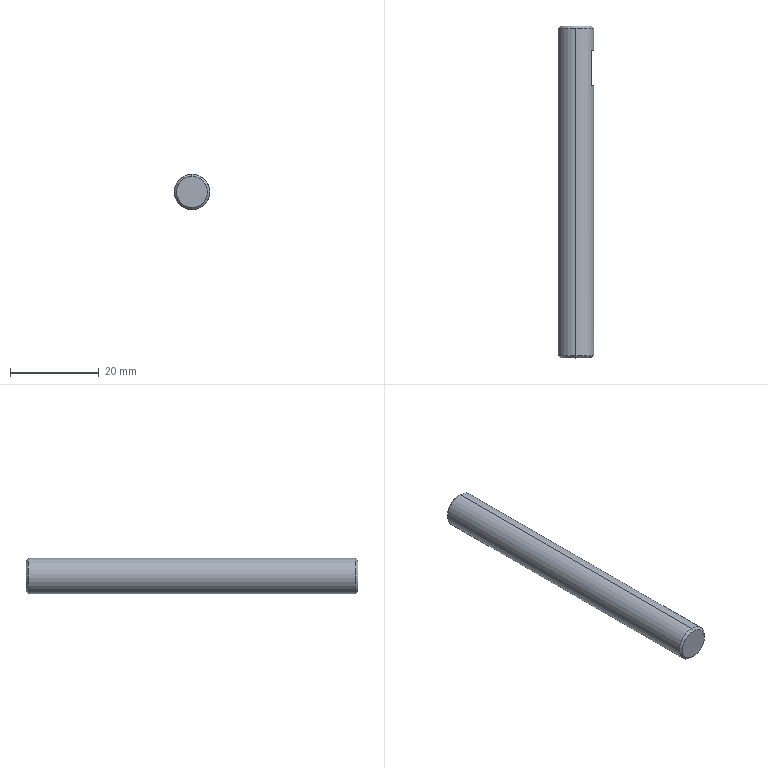Part | SolidWorks | features Chamfer 1, Extrusion 1, ICE 1 | 1 solid | 11 faces | box 8 x 75 x 8 mm | volume 3753 mm3 | plane 5 | cone 4 | cylinder 2 | commonest cylinder face diameters 8 x2
STEP:
#1=CARTESIAN_POINT('',(0.,75.,3.5));
#2=VERTEX_POINT('',#1);
#3=CARTESIAN_POINT('',(0.,75.,-3.5));
#4=VERTEX_POINT('',#3);
#5=CARTESIAN_POINT('',(0.,75.,0.));
#6=DIRECTION('',(0.,1.,0.));
#7=DIRECTION('',(0.,0.,1.));
#8=AXIS2_PLACEMENT_3D('',#5,#6,#7);
#9=CIRCLE('',#8,3.5);
#10=EDGE_CURVE('',#2,#4,#9,.T.);
#11=ORIENTED_EDGE('',*,*,#10,.F.);
#12=CARTESIAN_POINT('',(0.,74.5,4.));
#13=VERTEX_POINT('',#12);
#14=CARTESIAN_POINT('',(0.,75.,3.5));
#15=DIRECTION('',(0.,-0.7071,0.7071));
#16=VECTOR('',#15,1000.);
#17=LINE('',#14,#16);
#18=EDGE_CURVE('',#2,#13,#17,.T.);
#19=ORIENTED_EDGE('',*,*,#18,.T.);
#20=CARTESIAN_POINT('',(0.,74.5,-4.));
#21=VERTEX_POINT('',#20);
#22=CARTESIAN_POINT('',(0.,74.5,0.));
#23=DIRECTION('',(0.,-1.,0.));
#24=DIRECTION('',(0.,0.,1.));
#25=AXIS2_PLACEMENT_3D('',#22,#23,#24);
#26=CIRCLE('',#25,4.);
#27=EDGE_CURVE('',#21,#13,#26,.T.);
#28=ORIENTED_EDGE('',*,*,#27,.F.);
#29=CARTESIAN_POINT('',(0.,75.,-3.5));
#30=DIRECTION('',(0.,-0.7071,-0.7071));
#31=VECTOR('',#30,1000.);
#32=LINE('',#29,#31);
#33=EDGE_CURVE('',#4,#21,#32,.T.);
#34=ORIENTED_EDGE('',*,*,#33,.F.);
#35=EDGE_LOOP('',(#11,#19,#28,#34));
#36=FACE_OUTER_BOUND('',#35,.T.);
#37=CARTESIAN_POINT('',(0.,75.,0.));
#38=DIRECTION('',(0.,-1.,0.));
#39=DIRECTION('',(0.,0.,-1.));
#40=AXIS2_PLACEMENT_3D('',#37,#38,#39);
#41=CONICAL_SURFACE('',#40,3.5,0.7854);
#42=ADVANCED_FACE('',(#36),#41,.T.);
#43=CARTESIAN_POINT('',(0.,0.,-3.5));
#44=VERTEX_POINT('',#43);
#45=CARTESIAN_POINT('',(0.,0.,3.5));
#46=VERTEX_POINT('',#45);
#47=CARTESIAN_POINT('',(0.,0.,0.));
#48=DIRECTION('',(0.,-1.,0.));
#49=DIRECTION('',(0.,0.,1.));
#50=AXIS2_PLACEMENT_3D('',#47,#48,#49);
#51=CIRCLE('',#50,3.5);
#52=EDGE_CURVE('',#44,#46,#51,.T.);
#53=ORIENTED_EDGE('',*,*,#52,.F.);
#54=CARTESIAN_POINT('',(0.,0.5,-4.));
#55=VERTEX_POINT('',#54);
#56=CARTESIAN_POINT('',(0.,0.5,-4.));
#57=DIRECTION('',(0.,0.7071,-0.7071));
#58=VECTOR('',#57,1000.);
#59=LINE('',#56,#58);
#60=EDGE_CURVE('',#44,#55,#59,.T.);
#61=ORIENTED_EDGE('',*,*,#60,.T.);
#62=CARTESIAN_POINT('',(0.,0.5,4.));
#63=VERTEX_POINT('',#62);
#64=CARTESIAN_POINT('',(0.,0.5,0.));
#65=DIRECTION('',(0.,1.,0.));
#66=DIRECTION('',(0.,0.,1.));
#67=AXIS2_PLACEMENT_3D('',#64,#65,#66);
#68=CIRCLE('',#67,4.);
#69=EDGE_CURVE('',#63,#55,#68,.T.);
#70=ORIENTED_EDGE('',*,*,#69,.F.);
#71=CARTESIAN_POINT('',(0.,0.5,4.));
#72=DIRECTION('',(0.,0.7071,0.7071));
#73=VECTOR('',#72,1000.);
#74=LINE('',#71,#73);
#75=EDGE_CURVE('',#46,#63,#74,.T.);
#76=ORIENTED_EDGE('',*,*,#75,.F.);
#77=EDGE_LOOP('',(#53,#61,#70,#76));
#78=FACE_OUTER_BOUND('',#77,.T.);
#79=CARTESIAN_POINT('',(0.,0.5,0.));
#80=DIRECTION('',(0.,1.,0.));
#81=DIRECTION('',(0.,0.,1.));
#82=AXIS2_PLACEMENT_3D('',#79,#80,#81);
#83=CONICAL_SURFACE('',#82,4.,0.7854);
#84=ADVANCED_FACE('',(#78),#83,.T.);
#85=CARTESIAN_POINT('',(3.5,69.5,-1.936));
#86=VERTEX_POINT('',#85);
#87=CARTESIAN_POINT('',(3.5,61.5,-1.936));
#88=VERTEX_POINT('',#87);
#89=CARTESIAN_POINT('',(3.5,75.,-1.936));
#90=DIRECTION('',(0.,-1.,0.));
#91=VECTOR('',#90,1000.);
#92=LINE('',#89,#91);
#93=EDGE_CURVE('',#86,#88,#92,.T.);
#94=ORIENTED_EDGE('',*,*,#93,.T.);
#95=CARTESIAN_POINT('',(3.5,61.5,1.936));
#96=VERTEX_POINT('',#95);
#97=CARTESIAN_POINT('',(0.,61.5,0.));
#98=DIRECTION('',(0.,-1.,0.));
#99=DIRECTION('',(0.,0.,-1.));
#100=AXIS2_PLACEMENT_3D('',#97,#98,#99);
#101=CIRCLE('',#100,4.);
#102=EDGE_CURVE('',#88,#96,#101,.T.);
#103=ORIENTED_EDGE('',*,*,#102,.T.);
#104=CARTESIAN_POINT('',(3.5,69.5,1.936));
#105=VERTEX_POINT('',#104);
#106=CARTESIAN_POINT('',(3.5,75.,1.936));
#107=DIRECTION('',(0.,1.,0.));
#108=VECTOR('',#107,1000.);
#109=LINE('',#106,#108);
#110=EDGE_CURVE('',#96,#105,#109,.T.);
#111=ORIENTED_EDGE('',*,*,#110,.T.);
#112=CARTESIAN_POINT('',(0.,69.5,0.));
#113=DIRECTION('',(0.,1.,0.));
#114=DIRECTION('',(0.,0.,1.));
#115=AXIS2_PLACEMENT_3D('',#112,#113,#114);
#116=CIRCLE('',#115,4.);
#117=EDGE_CURVE('',#105,#86,#116,.T.);
#118=ORIENTED_EDGE('',*,*,#117,.T.);
#119=EDGE_LOOP('',(#94,#103,#111,#118));
#120=FACE_BOUND('',#119,.T.);
#121=ORIENTED_EDGE('',*,*,#27,.T.);
#122=CARTESIAN_POINT('',(0.,75.,4.));
#123=DIRECTION('',(0.,-1.,0.));
#124=VECTOR('',#123,1000.);
#125=LINE('',#122,#124);
#126=EDGE_CURVE('',#13,#63,#125,.T.);
#127=ORIENTED_EDGE('',*,*,#126,.T.);
#128=ORIENTED_EDGE('',*,*,#69,.T.);
#129=CARTESIAN_POINT('',(0.,75.,-4.));
#130=DIRECTION('',(0.,-1.,0.));
#131=VECTOR('',#130,1000.);
#132=LINE('',#129,#131);
#133=EDGE_CURVE('',#21,#55,#132,.T.);
#134=ORIENTED_EDGE('',*,*,#133,.F.);
#135=EDGE_LOOP('',(#121,#127,#128,#134));
#136=FACE_OUTER_BOUND('',#135,.T.);
#137=CARTESIAN_POINT('',(0.,75.,0.));
#138=DIRECTION('',(0.,-1.,0.));
#139=DIRECTION('',(0.,0.,-1.));
#140=AXIS2_PLACEMENT_3D('',#137,#138,#139);
#141=CYLINDRICAL_SURFACE('',#140,4.);
#142=ADVANCED_FACE('',(#120,#136),#141,.T.);
#143=ORIENTED_EDGE('',*,*,#126,.F.);
#144=CARTESIAN_POINT('',(0.,74.5,0.));
#145=DIRECTION('',(0.,-1.,0.));
#146=DIRECTION('',(0.,0.,1.));
#147=AXIS2_PLACEMENT_3D('',#144,#145,#146);
#148=CIRCLE('',#147,4.);
#149=EDGE_CURVE('',#13,#21,#148,.T.);
#150=ORIENTED_EDGE('',*,*,#149,.T.);
#151=ORIENTED_EDGE('',*,*,#133,.T.);
#152=CARTESIAN_POINT('',(0.,0.5,0.));
#153=DIRECTION('',(0.,1.,0.));
#154=DIRECTION('',(0.,0.,1.));
#155=AXIS2_PLACEMENT_3D('',#152,#153,#154);
#156=CIRCLE('',#155,4.);
#157=EDGE_CURVE('',#55,#63,#156,.T.);
#158=ORIENTED_EDGE('',*,*,#157,.T.);
#159=EDGE_LOOP('',(#143,#150,#151,#158));
#160=FACE_OUTER_BOUND('',#159,.T.);
#161=CARTESIAN_POINT('',(0.,75.,0.));
#162=DIRECTION('',(0.,-1.,0.));
#163=DIRECTION('',(0.,0.,-1.));
#164=AXIS2_PLACEMENT_3D('',#161,#162,#163);
#165=CYLINDRICAL_SURFACE('',#164,4.);
#166=ADVANCED_FACE('',(#160),#165,.T.);
#167=CARTESIAN_POINT('',(0.,75.,0.));
#168=DIRECTION('',(0.,1.,0.));
#169=DIRECTION('',(0.,0.,1.));
#170=AXIS2_PLACEMENT_3D('',#167,#168,#169);
#171=CIRCLE('',#170,3.5);
#172=EDGE_CURVE('',#4,#2,#171,.T.);
#173=ORIENTED_EDGE('',*,*,#172,.T.);
#174=ORIENTED_EDGE('',*,*,#10,.T.);
#175=EDGE_LOOP('',(#173,#174));
#176=FACE_OUTER_BOUND('',#175,.T.);
#177=CARTESIAN_POINT('',(0.,75.,0.));
#178=DIRECTION('',(0.,1.,0.));
#179=DIRECTION('',(0.,0.,1.));
#180=AXIS2_PLACEMENT_3D('',#177,#178,#179);
#181=PLANE('',#180);
#182=ADVANCED_FACE('',(#176),#181,.T.);
#183=CARTESIAN_POINT('',(0.,0.,0.));
#184=DIRECTION('',(0.,-1.,0.));
#185=DIRECTION('',(0.,0.,1.));
#186=AXIS2_PLACEMENT_3D('',#183,#184,#185);
#187=CIRCLE('',#186,3.5);
#188=EDGE_CURVE('',#46,#44,#187,.T.);
#189=ORIENTED_EDGE('',*,*,#188,.T.);
#190=ORIENTED_EDGE('',*,*,#52,.T.);
#191=EDGE_LOOP('',(#189,#190));
#192=FACE_OUTER_BOUND('',#191,.T.);
#193=CARTESIAN_POINT('',(0.,0.,0.));
#194=DIRECTION('',(0.,1.,0.));
#195=DIRECTION('',(0.,0.,1.));
#196=AXIS2_PLACEMENT_3D('',#193,#194,#195);
#197=PLANE('',#196);
#198=ADVANCED_FACE('',(#192),#197,.F.);
#199=ORIENTED_EDGE('',*,*,#60,.F.);
#200=ORIENTED_EDGE('',*,*,#188,.F.);
#201=ORIENTED_EDGE('',*,*,#75,.T.);
#202=ORIENTED_EDGE('',*,*,#157,.F.);
#203=EDGE_LOOP('',(#199,#200,#201,#202));
#204=FACE_OUTER_BOUND('',#203,.T.);
#205=CARTESIAN_POINT('',(0.,0.5,0.));
#206=DIRECTION('',(0.,1.,0.));
#207=DIRECTION('',(0.,0.,1.));
#208=AXIS2_PLACEMENT_3D('',#205,#206,#207);
#209=CONICAL_SURFACE('',#208,4.,0.7854);
#210=ADVANCED_FACE('',(#204),#209,.T.);
#211=ORIENTED_EDGE('',*,*,#18,.F.);
#212=ORIENTED_EDGE('',*,*,#172,.F.);
#213=ORIENTED_EDGE('',*,*,#33,.T.);
#214=ORIENTED_EDGE('',*,*,#149,.F.);
#215=EDGE_LOOP('',(#211,#212,#213,#214));
#216=FACE_OUTER_BOUND('',#215,.T.);
#217=CARTESIAN_POINT('',(0.,75.,0.));
#218=DIRECTION('',(0.,-1.,0.));
#219=DIRECTION('',(0.,0.,-1.));
#220=AXIS2_PLACEMENT_3D('',#217,#218,#219);
#221=CONICAL_SURFACE('',#220,3.5,0.7854);
#222=ADVANCED_FACE('',(#216),#221,.T.);
#223=CARTESIAN_POINT('',(3.5,61.5,-5.));
#224=DIRECTION('',(0.,0.,1.));
#225=VECTOR('',#224,1000.);
#226=LINE('',#223,#225);
#227=EDGE_CURVE('',#88,#96,#226,.T.);
#228=ORIENTED_EDGE('',*,*,#227,.T.);
#229=ORIENTED_EDGE('',*,*,#102,.F.);
#230=EDGE_LOOP('',(#228,#229));
#231=FACE_OUTER_BOUND('',#230,.T.);
#232=CARTESIAN_POINT('',(3.5,61.5,-5.));
#233=DIRECTION('',(0.,-1.,0.));
#234=DIRECTION('',(0.,0.,-1.));
#235=AXIS2_PLACEMENT_3D('',#232,#233,#234);
#236=PLANE('',#235);
#237=ADVANCED_FACE('',(#231),#236,.F.);
#238=CARTESIAN_POINT('',(3.5,69.5,-5.));
#239=DIRECTION('',(0.,0.,1.));
#240=VECTOR('',#239,1000.);
#241=LINE('',#238,#240);
#242=EDGE_CURVE('',#86,#105,#241,.T.);
#243=ORIENTED_EDGE('',*,*,#242,.T.);
#244=ORIENTED_EDGE('',*,*,#110,.F.);
#245=ORIENTED_EDGE('',*,*,#227,.F.);
#246=ORIENTED_EDGE('',*,*,#93,.F.);
#247=EDGE_LOOP('',(#243,#244,#245,#246));
#248=FACE_OUTER_BOUND('',#247,.T.);
#249=CARTESIAN_POINT('',(3.5,69.5,-5.));
#250=DIRECTION('',(-1.,0.,0.));
#251=DIRECTION('',(0.,0.,1.));
#252=AXIS2_PLACEMENT_3D('',#249,#250,#251);
#253=PLANE('',#252);
#254=ADVANCED_FACE('',(#248),#253,.F.);
#255=ORIENTED_EDGE('',*,*,#242,.F.);
#256=ORIENTED_EDGE('',*,*,#117,.F.);
#257=EDGE_LOOP('',(#255,#256));
#258=FACE_OUTER_BOUND('',#257,.T.);
#259=CARTESIAN_POINT('',(3.5,69.5,-5.));
#260=DIRECTION('',(0.,1.,0.));
#261=DIRECTION('',(0.,0.,1.));
#262=AXIS2_PLACEMENT_3D('',#259,#260,#261);
#263=PLANE('',#262);
#264=ADVANCED_FACE('',(#258),#263,.F.);
#265=CLOSED_SHELL('',(#42,#84,#142,#166,#182,#198,#210,#222,#237,#254,#264));
#266=MANIFOLD_SOLID_BREP('',#265);
#267=CARTESIAN_POINT('',(0.,0.,0.));
#268=DIRECTION('',(0.,0.,1.));
#269=DIRECTION('',(1.,0.,0.));
#270=AXIS2_PLACEMENT_3D('',#267,#268,#269);
#271=(LENGTH_UNIT()NAMED_UNIT(*)SI_UNIT(.MILLI.,.METRE.));
#272=UNCERTAINTY_MEASURE_WITH_UNIT(LENGTH_MEASURE(0.00001),#271,'','');
#273=(NAMED_UNIT(*)PLANE_ANGLE_UNIT()SI_UNIT($,.RADIAN.));
#274=(NAMED_UNIT(*)SI_UNIT($,.STERADIAN.)SOLID_ANGLE_UNIT());
#275=(GEOMETRIC_REPRESENTATION_CONTEXT(3)GLOBAL_UNCERTAINTY_ASSIGNED_CONTEXT((#272))GLOBAL_UNIT_ASSIGNED_CONTEXT((#271,#273,#274))REPRESENTATION_CONTEXT('',''));
#276=ADVANCED_BREP_SHAPE_REPRESENTATION('',(#266,#270),#275);